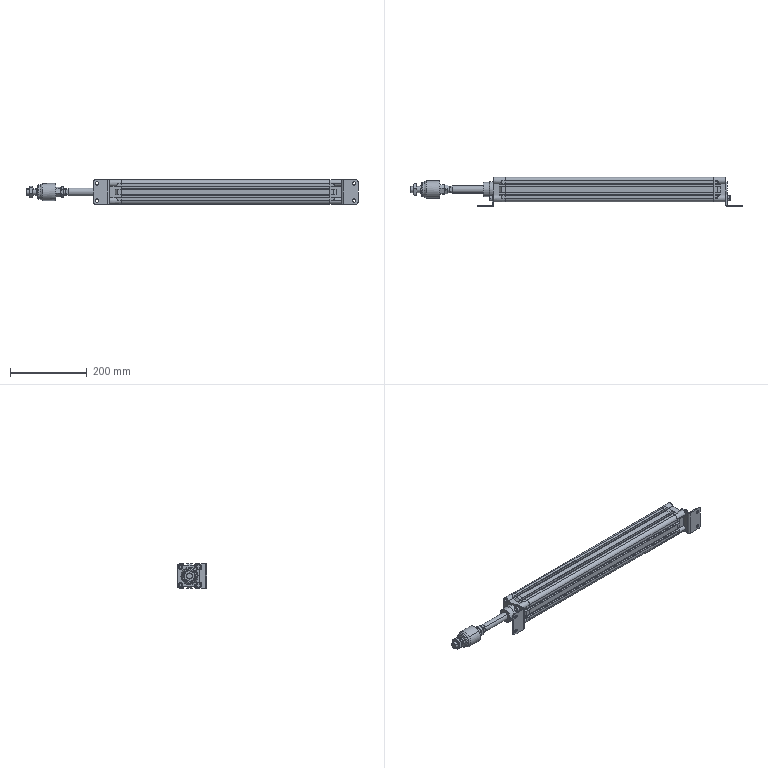Part | NX | features BREP 6 | 10 solids | 642 faces | box 865.361 x 77 x 65 mm | volume 1559018 mm3 | plane 277 | cylinder 261 | cone 92 | torus 12 | commonest cylinder face diameters 1 x102 6.647 x16 9 x16 12.4 x16 8 x10 17.5 x10